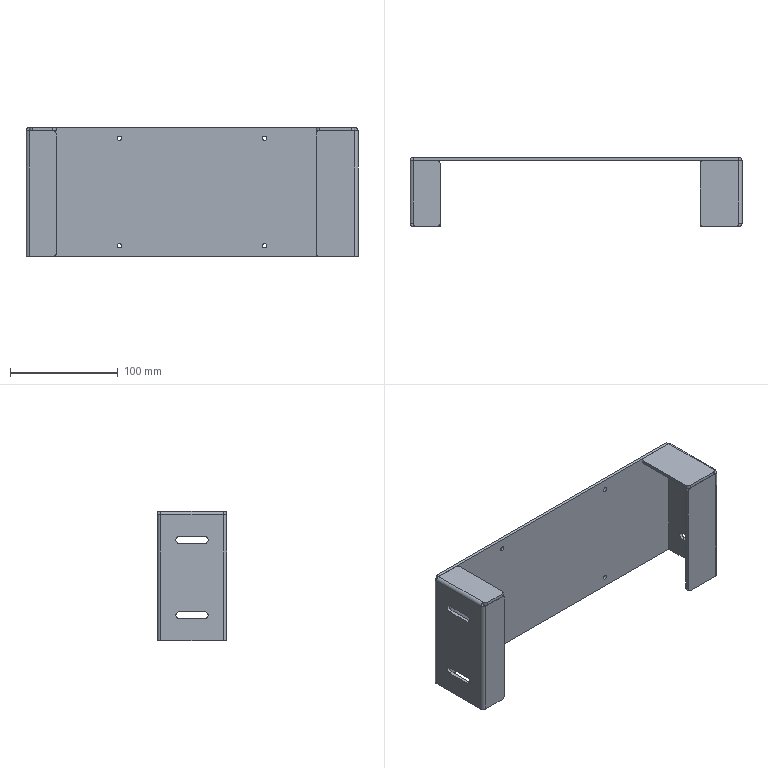Part | STEP file | 1 solid | 102 faces | box 308.5 x 64.5 x 120 mm | volume 184454 mm3 | plane 56 | cylinder 46 | commonest cylinder face diameters 6 x10 4 x8 6.5 x8 0.2 x6 6.2 x6 3.3 x4